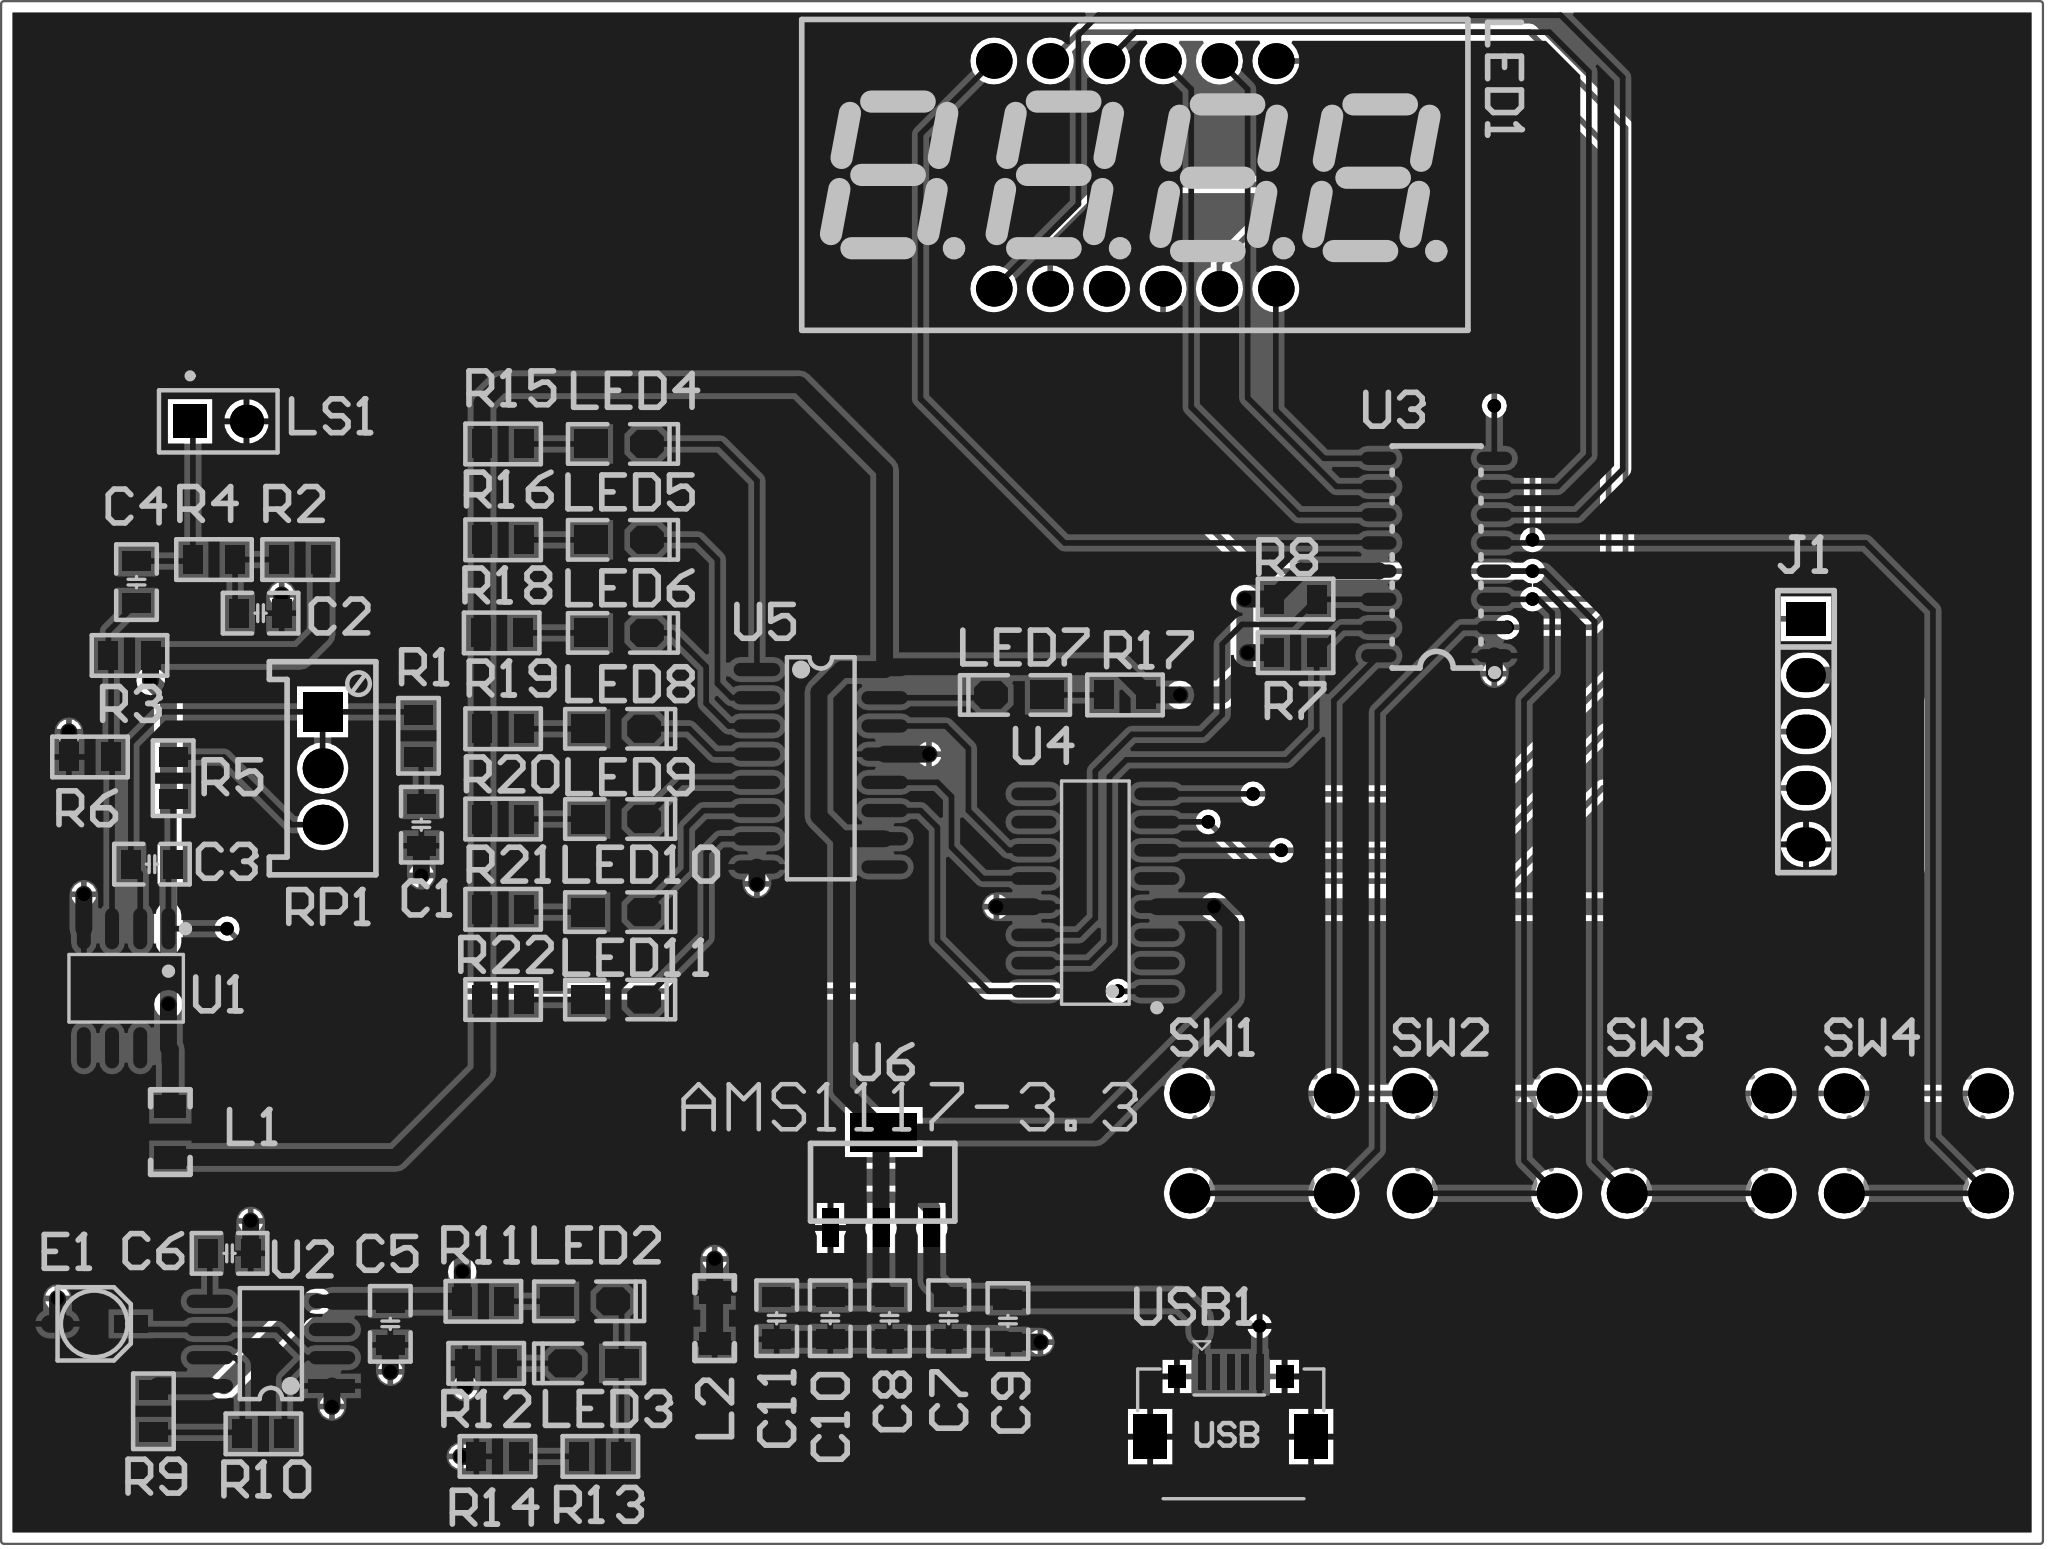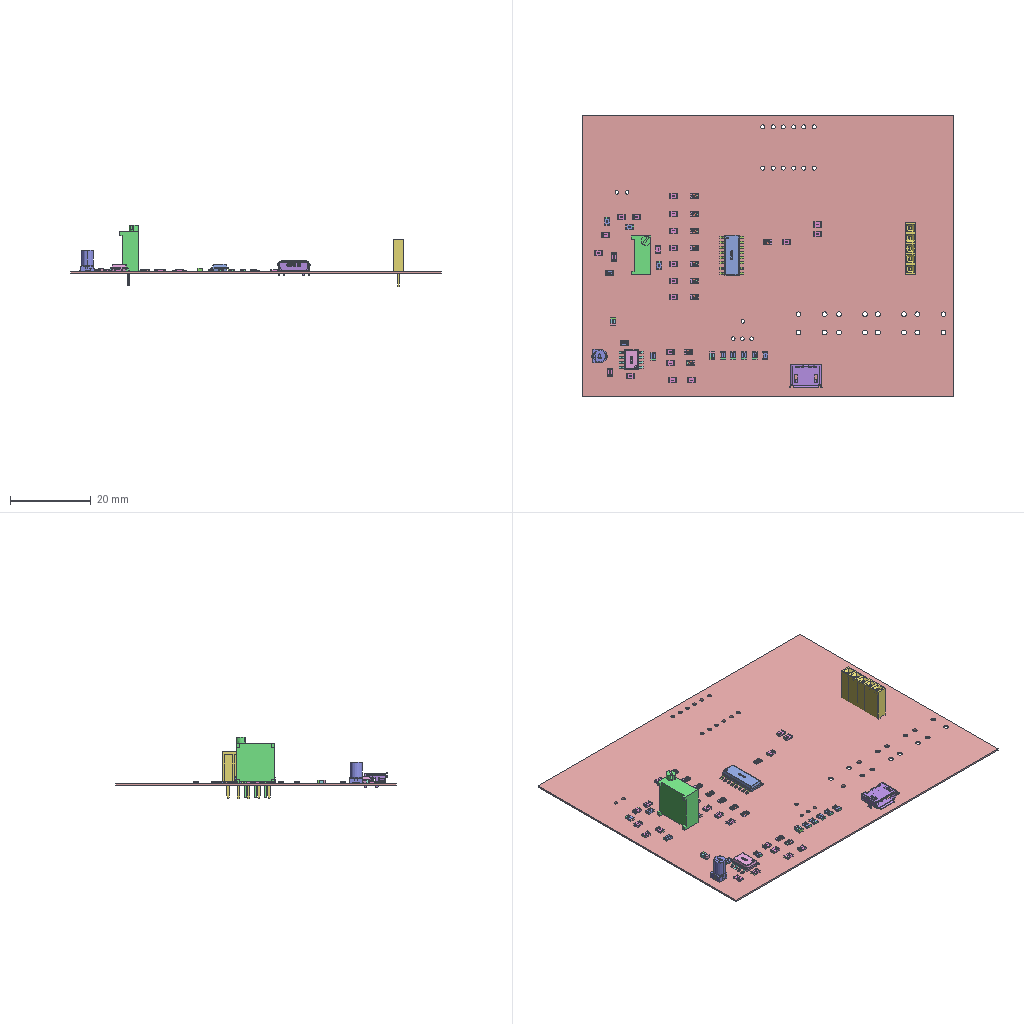Circuit board layout | Altium Designer | box 91.9 x 69.5 x 15.1 mm
Layer stack:
# Altium Designer layer stack of  (unit mm; dielectric type: 0 none, 1 core, 2 prepreg, 3 surface material)
index,name,kind,layer,copper_thickness_mm,dielectric_type,dielectric_thickness_mm,dielectric_material,dielectric_constant
0,Top Paste,other,,,,,,
1,Top Overlay,other,,,,,,
2,Top Solder,dielectric,,,3,0.0102,Solder Resist,3.5
3,Top Layer,copper,Top Layer,0.0356,,,,
4,Dielectric 1,dielectric,,,0,0.32,FR-4,4.8
5,Bottom Layer,copper,Bottom Layer,0.0356,,,,
6,Bottom Solder,dielectric,,,3,0.0102,Solder Resist,3.5
7,Bottom Overlay,other,,,,,,
8,Bottom Paste,other,,,,,,
# drill layer pairs: low layer,high layer
drill_pair,Top Layer,Bottom Layer
Part placement:
Designator,Comment,Layer,Footprint,Center-X(mm),Center-Y(mm),Rotation
U5,74HC595D,TopLayer,SOP16,132.669,69.723,0
U2,NE555,TopLayer,SOP8,107.906,43.815,180
USB1,USB-5P,TopLayer,USB-MICRO_A,151.13,41.074,0
U6,AMS1117-3.3,TopLayer,AMS1117-3.3,135.387,51.181,360
U4,PY32F002AW15S6TU,TopLayer,SOP-16_L9.9-W3.9-P1.27-LS6.0-BL,145.034,64.124,90
U3,GN1651,TopLayer,SOP-16_L9.9-W3.9-P1.27-LS6.1-BL,160.401,79.235,90
U1,COS2333SRC,TopLayer,SOP-8_L4.9-W3.9-P1.27-LS6.0-BL,101.388,59.817,180
SW4,6x6x5,TopLayer,四脚轻触开关,181.991,52.832,0
SW3,6x6x5,TopLayer,四脚轻触开关,172.212,52.832,0
SW2,6x6x5,TopLayer,四脚轻触开关,162.56,52.832,0
SW1,6x6x5,TopLayer,四脚轻触开关,152.527,52.832,0
RP1,10K,TopLayer,3296W,110.236,69.723,270
R22,1K,TopLayer,R_0805_L,118.364,59.309,360
R21,1K,TopLayer,R_0805_L,118.364,63.373,0
R20,1K,TopLayer,R_0805_L,118.364,67.437,360
R19,1K,TopLayer,R_0805_L,118.364,71.501,0
R18,1K,TopLayer,R_0805_L,118.298,75.819,0
R17,1K,TopLayer,R_0805_L,146.37,73.025,180
R16,1K,TopLayer,R_0805_L,118.364,80.01,0
R15,1K,TopLayer,R_0805_L,118.364,84.328,0
R14,25K,TopLayer,R_0805_L,118.11,38.735,180
R13,10K,TopLayer,R_0805_L,122.743,38.735,180
R12,1K,TopLayer,R_0805_L,117.602,42.926,180
R11,1K,TopLayer,R_0805_L,117.475,45.72,360
R10,200K,TopLayer,R_0805_L,107.569,39.751,180
R9,100K,TopLayer,R_0805_L,102.616,40.767,90
R8,10K,TopLayer,R_0805_L,154.051,77.343,180
R7,10K,TopLayer,R_0805_L,154.051,74.93,180
R6,1M,TopLayer,R_0805_L,99.761,70.231,180
R5,10K,TopLayer,R_0805_L,103.505,69.276,270
R4,1K,TopLayer,R_0805_L,105.344,79.121,360
R3,1M,TopLayer,R_0805_L,101.539,74.803,360
R2,1K,TopLayer,R_0805_L,109.22,79.121,360
R1,1K,TopLayer,R_0805_L,114.554,71.186,270
LS1,Bell,TopLayer,PIN2,105.537,85.344,360
LED11,Red,TopLayer,LED_0805G,123.444,59.309,360
LED10,Red,TopLayer,LED_0805G,123.444,63.246,360
LED9,Red,TopLayer,LED_0805G,123.444,67.437,360
LED8,Red,TopLayer,LED_0805G,123.444,71.501,360
LED7,Red,TopLayer,LED_0805G,141.605,73.025,180
LED6,Red,TopLayer,LED_0805G,123.571,75.819,360
LED5,Red,TopLayer,LED_0805G,123.571,80.01,360
LED4,Red,TopLayer,LED_0805G,123.571,84.328,360
LED3,Red,TopLayer,LED_0805G,122.428,42.926,180
LED2,Red,TopLayer,LED_0805G,122.047,45.72,360
LED1,SR410361N,TopLayer,LED-SEG-TH_12P-L30.0-W14.0-P2.54-S10.26-BL,146.812,96.443,360
L2,10uH,TopLayer,L_0805,127.889,44.958,90
L1,10uH,TopLayer,L_0805,103.378,53.34,270
J1,Female HDR1X5,TopLayer,Fe-HDR1X5/2.54-S,177.038,71.374,360
E1,10uF,TopLayer,CM_A(3*5.4),99.95,44.704,360
C11,100NF,TopLayer,C_0805_L,130.683,44.958,90
C10,10UF,TopLayer,C_0805_L,133.096,44.958,90
C9,10UF,TopLayer,C_0805_L,141.097,44.831,90
C8,100NF,TopLayer,C_0805_L,135.763,44.958,90
C7,100NF,TopLayer,C_0805_L,138.43,44.958,90
C6,10NF,TopLayer,C_0805_L,106.045,47.879,360
C5,10UF,TopLayer,C_0805_L,113.284,44.704,90
C4,0.01UF,TopLayer,C_0805_L,101.854,78.105,270
C3,100PF,TopLayer,C_0805_L,102.55,65.405,360
C2,0.1UF,TopLayer,C_0805_L,107.442,76.708,180
C1,10UF,TopLayer,C_0805_L,114.681,67.183,270
Pad and via stacks:
# Altium Designer via and pad stacks of  (unit mm). Each distinct definition once, with the count of objects using it.
# via: kind,start_layer,end_layer,hole_mm,diameter_mm,mode(0 simple;1 top-mid-bottom;2 full stack),diameter_per_layer,count,example_net
# pad: kind,layer,hole_mm,hole_type(0 round;1 square;2 slot),plating,top_size,top_shape(1 round;2 rect;3 octagon;9 rounded rect),mid_size,bottom_size,mode,footprint,size_per_layer,count,example
pad,Top Layer,0,0,plated,0.6x2.1,1,0.6x2.1,0.6x2.1,0,SOP16,,16,U5.1
pad,Top Layer,0,0,plated,0.6x2.1,1,0.6x2.1,0.6x2.1,0,SOP8,,7,U2.5
pad,Top Layer,0,0,plated,0.6x2.1,2,0.6x2.1,0.6x2.1,0,SOP8,,1,U2.1
pad,Top Layer,0,0,plated,1.27x0.889,2,1.27x0.889,1.27x0.889,0,C 0805_L,,22,C1.1
pad,Top Layer,0,0,plated,1.27x0.889,2,1.27x0.889,1.27x0.889,0,R 0805_L,,44,R1.1
pad,Top Layer,0,0,plated,0.63x1.865,1,0.63x1.865,0.63x1.865,0,SOP-8_L4.9-W3.9-P1.27-LS6.0-BL,,8,U1.5
pad,Top Layer,0,0,plated,1.5x0.8,2,1.5x0.8,1.5x0.8,0,CM A(3*5.4),,1,E1.1
pad,Top Layer,0,0,plated,1.5x0.8,1,1.5x0.8,1.5x0.8,0,CM A(3*5.4),,1,E1.2
pad,Top Layer,0,0,plated,0.6x1.6,1,0.6x1.6,0.6x1.6,0,SOP-16_L9.9-W3.9-P1.27-LS6.1-BL,,16,U3.1
pad,Top Layer,0,0,plated,1.524x1.27,2,1.524x1.27,1.524x1.27,0,LED 0805G,,10,LED3.1
pad,Top Layer,0,0,plated,1.524x1.27,3,1.524x1.27,1.524x1.27,0,LED 0805G,,10,LED3.2
pad,Top Layer,0,0,plated,0.574x2.038,1,0.574x2.038,0.574x2.038,0,SOP-16_L9.9-W3.9-P1.27-LS6.0-BL,,16,U4.1
pad,Top Layer,0,0,plated,1.6x0.35,2,1.6x0.35,1.6x0.35,0,USB-MICRO_A,,5,USB1.2
pad,Top Layer,0,0,plated,1.016x1.397,2,1.016x1.397,1.016x1.397,0,L 0805,,4,L1.2
pad,Multi-Layer,1,0,plated,1.6x1.6,1,1.6x1.6,1.6x1.6,0,LED-SEG-TH_12P-L30.0-W14.0-P2.54-S10.26-BL,,12,LED1.12
pad,Multi-Layer,0.7,0,plated,1.8x1.8,1,1.8x1.8,1.8x1.8,0,3296W,,2,RP1.3
pad,Multi-Layer,0.7,0,plated,1.8x1.8,2,1.8x1.8,1.8x1.8,0,3296W,,1,RP1.1
pad,Multi-Layer,0.9,0,plated,1.5x1.5,2,1.5x1.5,1.5x1.5,0,PIN2,,1,LS1.1
pad,Multi-Layer,0.9,0,plated,1.5x1.5,1,1.5x1.5,1.5x1.5,0,PIN2,,1,LS1.2
pad,Multi-Layer,1.2,0,plated,1.8x1.8,1,1.8x1.8,1.8x1.8,0,\u00CB\u00C4\u00BD\u00C5\u00C7\u00E1\u00B4\u00A5\u00BF\u00AA\u00B9\u00D8,,16,SW1.1
pad,Multi-Layer,0.8128,0,plated,1.524x1.778,2,1.524x1.778,1.524x1.778,0,Fe-HDR1X5/2.54-S,,1,J1.1
pad,Multi-Layer,0.8128,0,plated,1.524x1.778,1,1.524x1.778,1.524x1.778,0,Fe-HDR1X5/2.54-S,,4,J1.2
pad,Multi-Layer,0.9144,0,plated,3x1.75,2,3x1.75,3x1.75,0,AMS1117-3.3,,1,U6.4
pad,Multi-Layer,0.9144,0,plated,0.74x1.75,2,0.74x1.75,0.74x1.75,0,AMS1117-3.3,,3,U6.3
pad,Multi-Layer,0.5,2,plated,1.5x2,2,1.5x2,1.5x2,0,USB-MICRO_A,,2,USB1.5
pad,Multi-Layer,0.5,0,plated,0.8x1,2,0.8x1,0.8x1,0,USB-MICRO_A,,2,USB1.5
via,Top Layer,Bottom Layer,0.3048,0.6096,0,,36,GND
Copper pours:
name,layer,net,type(0 solid;1 hatched;2 none)
D,Bottom Layer,GND,0
D,Top Layer,GND,0
Design rules, without the lines most boards share:
# Altium Designer design rules of  (exported by Altium Designer, unit mm)
# columns: name | kind | enabled | priority | scope1 | scope2 | descriptor | typed fields (field=value)
Clearance | 0 | enabled | 1 | All | All | Clearance Constraint (Gap=10mil) (All),(All) | gap=0.254
PlaneConnect | 6 | enabled | 1 | All | All | Power Plane Connect Rule(Relief Connect )(Expansion=20mil) (Conductor Width=10mil) (Air Gap=10mil) (Entries=4) (All) | relief_conductor_width=0.254 relief_entries=4 relief_expansion=0.508
PolygonConnect | 20 | enabled | 1 | All | All | Polygon Connect Rule(Relief Connect )(Conductor Width=10mil) (Relief Angle=90 Angle) (Entries=4) (Air Gap Width=10mil) (All),(All) | connect_style(0=relief,1=direct,2=none)=0 relief_conductor_width=0.254 relief_entries=4
Width | 2 | enabled | 1 | All | All | Width Constraint (Min=10mil) (Max=30mil) (Preferred=10mil) (All) |
RoutingVias | 11 | enabled | 1 | All | All | Routing Via (MinHoleWidth=28mil) (MaxHoleWidth=28mil) (PreferredHoleWidth=28mil) (MinWidth=50mil) (MaxWidth=50mil) (PreferedWidth=50mil) (All) | via_min_hole=0.7112 via_max_hole=0.7112 via_preferred_diameter=1.27 via_preferred_hole=0.7112
PasteMaskExpansion | 14 | enabled | 1 | All | All | Paste Mask Expansion (Expansion =0mil) (All) | expansion=0
SolderMaskExpansion | 13 | enabled | 1 | All | All | Solder Mask Expansion (Expansion =4mil) (All) | expansion=0.1016
DiffPairsRouting | 51 | enabled | 1 | All | All | Differential Pairs Uncoupled Length using the Gap Constraints (Min=10mil) (Max=10mil) (Prefered=10mil)  and Width Constraints (Min=15mil) (Max=15mil) (Prefered=15mil) (All) |
HoleToHoleClearance | 52 | enabled | 1 | All | All | Hole To Hole Clearance (Gap=10mil) (All),(All) | gap=0.254
MinimumSolderMaskSliver | 53 | enabled | 1 | All | All | Minimum Solder Mask Sliver (Gap=0mil) (All),(All) |
SilkToSolderMaskClearance | 54 | enabled | 1 | IsPad | All | Silk To Solder Mask (Clearance=0mil) (IsPad),(All) |
SilkToSilkClearance | 55 | enabled | 1 | All | All | Silk to Silk (Clearance=0mil) (All),(All) |
Classes set for this board:
# Altium Designer classes of  (member kind: 0 net, 1 component, 2 from-to, 3 pad, 4 layer, 5 differential pair, 6 design channel, 7 polygon, 8 structure, 9 xSignal)
# columns: class name | member kind | superclass | members
Sheet1 | 1 | no | C1; C2; C3; C4; C5; C6; C7; C8; C9; C10; C11; E1; J1; L1; L2; LED1; LED2; LED3; LED4; LED5; LED6; LED7; LED8; LED9; LED10; LED11; LS1; R1; R2; R3; R4; R5; R6; R7; R8; R9; R10; R11; R12; R13; R14; R15; R16; R17; R18; R19; R20; R21; R22; RP1; SW1; SW2; SW3; SW4; U1; U2; U3; U4; U5; U6; USB1; U2; U5;